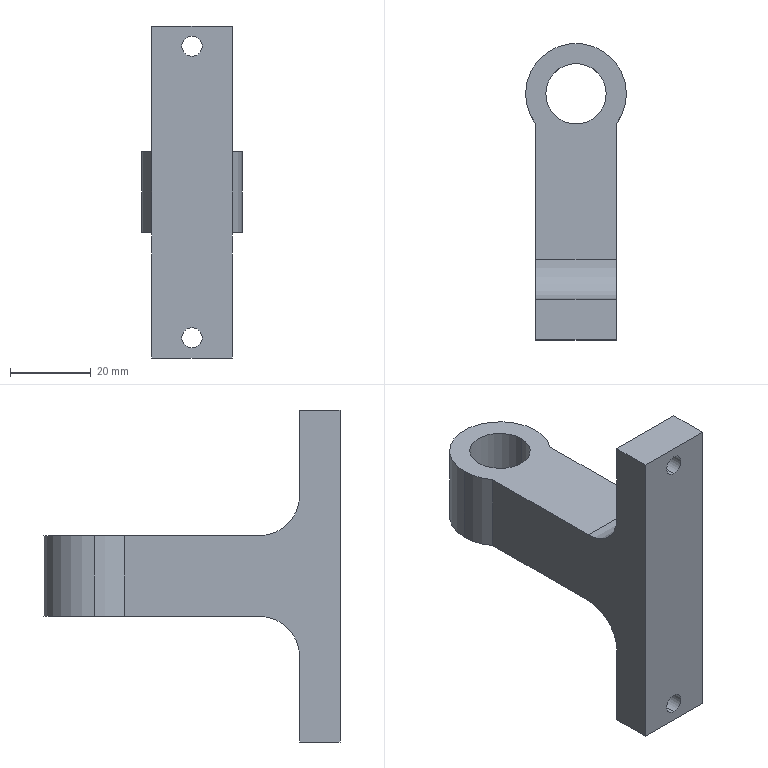Part | SolidWorks | features ICE 2, 3DProfileFeature 1, Extrusion 1, HoleWzd 1, MirrorPattern 1 | 1 solid | 20 faces | box 25 x 73.5 x 82.337 mm | volume 39218 mm3 | cylinder 11 | plane 9 | commonest cylinder face diameters 5 x4 25 x3 15 x2 20 x2
STEP:
#1=CARTESIAN_POINT('',(0.,-61.,-38.668));
#2=VERTEX_POINT('',#1);
#3=CARTESIAN_POINT('',(0.,-61.,-33.668));
#4=VERTEX_POINT('',#3);
#5=CARTESIAN_POINT('',(0.,-61.,-36.168));
#6=DIRECTION('',(0.,1.,0.));
#7=DIRECTION('',(0.,0.,1.));
#8=AXIS2_PLACEMENT_3D('',#5,#6,#7);
#9=CIRCLE('',#8,2.5);
#10=EDGE_CURVE('',#2,#4,#9,.T.);
#11=ORIENTED_EDGE('',*,*,#10,.F.);
#12=CARTESIAN_POINT('',(0.,-51.,-38.668));
#13=VERTEX_POINT('',#12);
#14=CARTESIAN_POINT('',(0.,-51.,-38.668));
#15=DIRECTION('',(0.,1.,0.));
#16=VECTOR('',#15,1000.);
#17=LINE('',#14,#16);
#18=EDGE_CURVE('',#2,#13,#17,.T.);
#19=ORIENTED_EDGE('',*,*,#18,.T.);
#20=CARTESIAN_POINT('',(0.,-51.,-33.668));
#21=VERTEX_POINT('',#20);
#22=CARTESIAN_POINT('',(0.,-51.,-36.168));
#23=DIRECTION('',(0.,1.,0.));
#24=DIRECTION('',(0.,0.,1.));
#25=AXIS2_PLACEMENT_3D('',#22,#23,#24);
#26=CIRCLE('',#25,2.5);
#27=EDGE_CURVE('',#13,#21,#26,.T.);
#28=ORIENTED_EDGE('',*,*,#27,.T.);
#29=CARTESIAN_POINT('',(0.,-51.,-33.668));
#30=DIRECTION('',(0.,1.,0.));
#31=VECTOR('',#30,1000.);
#32=LINE('',#29,#31);
#33=EDGE_CURVE('',#4,#21,#32,.T.);
#34=ORIENTED_EDGE('',*,*,#33,.F.);
#35=EDGE_LOOP('',(#11,#19,#28,#34));
#36=FACE_OUTER_BOUND('',#35,.T.);
#37=CARTESIAN_POINT('',(0.,-51.,-36.168));
#38=DIRECTION('',(0.,1.,0.));
#39=DIRECTION('',(0.,0.,1.));
#40=AXIS2_PLACEMENT_3D('',#37,#38,#39);
#41=CYLINDRICAL_SURFACE('',#40,2.5);
#42=ADVANCED_FACE('',(#36),#41,.F.);
#43=CARTESIAN_POINT('',(0.,-61.,33.668));
#44=VERTEX_POINT('',#43);
#45=CARTESIAN_POINT('',(0.,-61.,38.668));
#46=VERTEX_POINT('',#45);
#47=CARTESIAN_POINT('',(0.,-61.,36.168));
#48=DIRECTION('',(0.,1.,0.));
#49=DIRECTION('',(0.,0.,1.));
#50=AXIS2_PLACEMENT_3D('',#47,#48,#49);
#51=CIRCLE('',#50,2.5);
#52=EDGE_CURVE('',#44,#46,#51,.T.);
#53=ORIENTED_EDGE('',*,*,#52,.F.);
#54=CARTESIAN_POINT('',(0.,-51.,33.668));
#55=VERTEX_POINT('',#54);
#56=CARTESIAN_POINT('',(0.,-51.,33.668));
#57=DIRECTION('',(0.,1.,0.));
#58=VECTOR('',#57,1000.);
#59=LINE('',#56,#58);
#60=EDGE_CURVE('',#44,#55,#59,.T.);
#61=ORIENTED_EDGE('',*,*,#60,.T.);
#62=CARTESIAN_POINT('',(0.,-51.,38.668));
#63=VERTEX_POINT('',#62);
#64=CARTESIAN_POINT('',(0.,-51.,36.168));
#65=DIRECTION('',(0.,1.,0.));
#66=DIRECTION('',(0.,0.,1.));
#67=AXIS2_PLACEMENT_3D('',#64,#65,#66);
#68=CIRCLE('',#67,2.5);
#69=EDGE_CURVE('',#55,#63,#68,.T.);
#70=ORIENTED_EDGE('',*,*,#69,.T.);
#71=CARTESIAN_POINT('',(0.,-51.,38.668));
#72=DIRECTION('',(0.,1.,0.));
#73=VECTOR('',#72,1000.);
#74=LINE('',#71,#73);
#75=EDGE_CURVE('',#46,#63,#74,.T.);
#76=ORIENTED_EDGE('',*,*,#75,.F.);
#77=EDGE_LOOP('',(#53,#61,#70,#76));
#78=FACE_OUTER_BOUND('',#77,.T.);
#79=CARTESIAN_POINT('',(0.,-51.,36.168));
#80=DIRECTION('',(0.,1.,0.));
#81=DIRECTION('',(0.,0.,1.));
#82=AXIS2_PLACEMENT_3D('',#79,#80,#81);
#83=CYLINDRICAL_SURFACE('',#82,2.5);
#84=ADVANCED_FACE('',(#78),#83,.F.);
#85=CARTESIAN_POINT('',(-7.5,0.,10.));
#86=VERTEX_POINT('',#85);
#87=CARTESIAN_POINT('',(7.5,0.,10.));
#88=VERTEX_POINT('',#87);
#89=CARTESIAN_POINT('',(0.,0.,10.));
#90=DIRECTION('',(0.,0.,1.));
#91=DIRECTION('',(1.,0.,0.));
#92=AXIS2_PLACEMENT_3D('',#89,#90,#91);
#93=CIRCLE('',#92,7.5);
#94=EDGE_CURVE('',#86,#88,#93,.T.);
#95=ORIENTED_EDGE('',*,*,#94,.T.);
#96=CARTESIAN_POINT('',(7.5,0.,-10.));
#97=VERTEX_POINT('',#96);
#98=CARTESIAN_POINT('',(7.5,0.,10.));
#99=DIRECTION('',(0.,0.,-1.));
#100=VECTOR('',#99,1000.);
#101=LINE('',#98,#100);
#102=EDGE_CURVE('',#88,#97,#101,.T.);
#103=ORIENTED_EDGE('',*,*,#102,.T.);
#104=CARTESIAN_POINT('',(-7.5,0.,-10.));
#105=VERTEX_POINT('',#104);
#106=CARTESIAN_POINT('',(0.,0.,-10.));
#107=DIRECTION('',(0.,0.,1.));
#108=DIRECTION('',(1.,0.,0.));
#109=AXIS2_PLACEMENT_3D('',#106,#107,#108);
#110=CIRCLE('',#109,7.5);
#111=EDGE_CURVE('',#105,#97,#110,.T.);
#112=ORIENTED_EDGE('',*,*,#111,.F.);
#113=CARTESIAN_POINT('',(-7.5,0.,10.));
#114=DIRECTION('',(0.,0.,-1.));
#115=VECTOR('',#114,1000.);
#116=LINE('',#113,#115);
#117=EDGE_CURVE('',#86,#105,#116,.T.);
#118=ORIENTED_EDGE('',*,*,#117,.F.);
#119=EDGE_LOOP('',(#95,#103,#112,#118));
#120=FACE_OUTER_BOUND('',#119,.T.);
#121=CARTESIAN_POINT('',(0.,0.,10.));
#122=DIRECTION('',(0.,0.,-1.));
#123=DIRECTION('',(-1.,0.,0.));
#124=AXIS2_PLACEMENT_3D('',#121,#122,#123);
#125=CYLINDRICAL_SURFACE('',#124,7.5);
#126=ADVANCED_FACE('',(#120),#125,.F.);
#127=CARTESIAN_POINT('',(12.5,0.,10.));
#128=VERTEX_POINT('',#127);
#129=CARTESIAN_POINT('',(-12.5,0.,10.));
#130=VERTEX_POINT('',#129);
#131=CARTESIAN_POINT('',(0.,0.,10.));
#132=DIRECTION('',(0.,0.,1.));
#133=DIRECTION('',(1.,0.,0.));
#134=AXIS2_PLACEMENT_3D('',#131,#132,#133);
#135=CIRCLE('',#134,12.5);
#136=EDGE_CURVE('',#128,#130,#135,.T.);
#137=ORIENTED_EDGE('',*,*,#136,.F.);
#138=CARTESIAN_POINT('',(12.5,0.,-10.));
#139=VERTEX_POINT('',#138);
#140=CARTESIAN_POINT('',(12.5,0.,10.));
#141=DIRECTION('',(0.,0.,-1.));
#142=VECTOR('',#141,1000.);
#143=LINE('',#140,#142);
#144=EDGE_CURVE('',#128,#139,#143,.T.);
#145=ORIENTED_EDGE('',*,*,#144,.T.);
#146=CARTESIAN_POINT('',(-12.5,0.,-10.));
#147=VERTEX_POINT('',#146);
#148=CARTESIAN_POINT('',(0.,0.,-10.));
#149=DIRECTION('',(0.,0.,1.));
#150=DIRECTION('',(1.,0.,0.));
#151=AXIS2_PLACEMENT_3D('',#148,#149,#150);
#152=CIRCLE('',#151,12.5);
#153=EDGE_CURVE('',#139,#147,#152,.T.);
#154=ORIENTED_EDGE('',*,*,#153,.T.);
#155=CARTESIAN_POINT('',(-12.5,0.,10.));
#156=DIRECTION('',(0.,0.,-1.));
#157=VECTOR('',#156,1000.);
#158=LINE('',#155,#157);
#159=EDGE_CURVE('',#130,#147,#158,.T.);
#160=ORIENTED_EDGE('',*,*,#159,.F.);
#161=EDGE_LOOP('',(#137,#145,#154,#160));
#162=FACE_OUTER_BOUND('',#161,.T.);
#163=CARTESIAN_POINT('',(0.,0.,10.));
#164=DIRECTION('',(0.,0.,-1.));
#165=DIRECTION('',(-1.,0.,0.));
#166=AXIS2_PLACEMENT_3D('',#163,#164,#165);
#167=CYLINDRICAL_SURFACE('',#166,12.5);
#168=ADVANCED_FACE('',(#162),#167,.T.);
#169=CARTESIAN_POINT('',(-10.,-7.5,10.));
#170=VERTEX_POINT('',#169);
#171=CARTESIAN_POINT('',(0.,0.,10.));
#172=DIRECTION('',(0.,0.,1.));
#173=DIRECTION('',(1.,0.,0.));
#174=AXIS2_PLACEMENT_3D('',#171,#172,#173);
#175=CIRCLE('',#174,12.5);
#176=EDGE_CURVE('',#130,#170,#175,.T.);
#177=ORIENTED_EDGE('',*,*,#176,.F.);
#178=ORIENTED_EDGE('',*,*,#159,.T.);
#179=CARTESIAN_POINT('',(-10.,-7.5,-10.));
#180=VERTEX_POINT('',#179);
#181=CARTESIAN_POINT('',(0.,0.,-10.));
#182=DIRECTION('',(0.,0.,1.));
#183=DIRECTION('',(1.,0.,0.));
#184=AXIS2_PLACEMENT_3D('',#181,#182,#183);
#185=CIRCLE('',#184,12.5);
#186=EDGE_CURVE('',#147,#180,#185,.T.);
#187=ORIENTED_EDGE('',*,*,#186,.T.);
#188=CARTESIAN_POINT('',(-10.,-7.5,10.));
#189=DIRECTION('',(0.,0.,1.));
#190=VECTOR('',#189,1000.);
#191=LINE('',#188,#190);
#192=EDGE_CURVE('',#180,#170,#191,.T.);
#193=ORIENTED_EDGE('',*,*,#192,.T.);
#194=EDGE_LOOP('',(#177,#178,#187,#193));
#195=FACE_OUTER_BOUND('',#194,.T.);
#196=CARTESIAN_POINT('',(0.,0.,10.));
#197=DIRECTION('',(0.,0.,-1.));
#198=DIRECTION('',(-1.,0.,0.));
#199=AXIS2_PLACEMENT_3D('',#196,#197,#198);
#200=CYLINDRICAL_SURFACE('',#199,12.5);
#201=ADVANCED_FACE('',(#195),#200,.T.);
#202=CARTESIAN_POINT('',(-10.,-51.,-41.168));
#203=VERTEX_POINT('',#202);
#204=CARTESIAN_POINT('',(-10.,-51.,-20.));
#205=VERTEX_POINT('',#204);
#206=CARTESIAN_POINT('',(-10.,-51.,-20.));
#207=DIRECTION('',(0.,0.,1.));
#208=VECTOR('',#207,1000.);
#209=LINE('',#206,#208);
#210=EDGE_CURVE('',#203,#205,#209,.T.);
#211=ORIENTED_EDGE('',*,*,#210,.T.);
#212=CARTESIAN_POINT('',(10.,-51.,-20.));
#213=VERTEX_POINT('',#212);
#214=CARTESIAN_POINT('',(10.,-51.,-20.));
#215=DIRECTION('',(-1.,0.,0.));
#216=VECTOR('',#215,1000.);
#217=LINE('',#214,#216);
#218=EDGE_CURVE('',#213,#205,#217,.T.);
#219=ORIENTED_EDGE('',*,*,#218,.F.);
#220=CARTESIAN_POINT('',(10.,-51.,-41.168));
#221=VERTEX_POINT('',#220);
#222=CARTESIAN_POINT('',(10.,-51.,-21.658));
#223=DIRECTION('',(0.,0.,1.));
#224=VECTOR('',#223,1000.);
#225=LINE('',#222,#224);
#226=EDGE_CURVE('',#221,#213,#225,.T.);
#227=ORIENTED_EDGE('',*,*,#226,.F.);
#228=CARTESIAN_POINT('',(10.,-51.,-41.168));
#229=DIRECTION('',(-1.,0.,0.));
#230=VECTOR('',#229,1000.);
#231=LINE('',#228,#230);
#232=EDGE_CURVE('',#221,#203,#231,.T.);
#233=ORIENTED_EDGE('',*,*,#232,.T.);
#234=EDGE_LOOP('',(#211,#219,#227,#233));
#235=FACE_OUTER_BOUND('',#234,.T.);
#236=CARTESIAN_POINT('',(0.,-51.,-36.168));
#237=DIRECTION('',(0.,1.,0.));
#238=DIRECTION('',(0.,0.,1.));
#239=AXIS2_PLACEMENT_3D('',#236,#237,#238);
#240=CIRCLE('',#239,2.5);
#241=EDGE_CURVE('',#21,#13,#240,.T.);
#242=ORIENTED_EDGE('',*,*,#241,.F.);
#243=ORIENTED_EDGE('',*,*,#27,.F.);
#244=EDGE_LOOP('',(#242,#243));
#245=FACE_BOUND('',#244,.T.);
#246=CARTESIAN_POINT('',(10.,-51.,-20.));
#247=DIRECTION('',(0.,-1.,0.));
#248=DIRECTION('',(0.,0.,-1.));
#249=AXIS2_PLACEMENT_3D('',#246,#247,#248);
#250=PLANE('',#249);
#251=ADVANCED_FACE('',(#235,#245),#250,.F.);
#252=ORIENTED_EDGE('',*,*,#144,.F.);
#253=CARTESIAN_POINT('',(10.,-7.5,10.));
#254=VERTEX_POINT('',#253);
#255=CARTESIAN_POINT('',(0.,0.,10.));
#256=DIRECTION('',(0.,0.,1.));
#257=DIRECTION('',(1.,0.,0.));
#258=AXIS2_PLACEMENT_3D('',#255,#256,#257);
#259=CIRCLE('',#258,12.5);
#260=EDGE_CURVE('',#254,#128,#259,.T.);
#261=ORIENTED_EDGE('',*,*,#260,.F.);
#262=CARTESIAN_POINT('',(10.,-7.5,-10.));
#263=VERTEX_POINT('',#262);
#264=CARTESIAN_POINT('',(10.,-7.5,10.));
#265=DIRECTION('',(0.,0.,-1.));
#266=VECTOR('',#265,1000.);
#267=LINE('',#264,#266);
#268=EDGE_CURVE('',#254,#263,#267,.T.);
#269=ORIENTED_EDGE('',*,*,#268,.T.);
#270=CARTESIAN_POINT('',(0.,0.,-10.));
#271=DIRECTION('',(0.,0.,1.));
#272=DIRECTION('',(1.,0.,0.));
#273=AXIS2_PLACEMENT_3D('',#270,#271,#272);
#274=CIRCLE('',#273,12.5);
#275=EDGE_CURVE('',#263,#139,#274,.T.);
#276=ORIENTED_EDGE('',*,*,#275,.T.);
#277=EDGE_LOOP('',(#252,#261,#269,#276));
#278=FACE_OUTER_BOUND('',#277,.T.);
#279=CARTESIAN_POINT('',(0.,0.,10.));
#280=DIRECTION('',(0.,0.,-1.));
#281=DIRECTION('',(-1.,0.,0.));
#282=AXIS2_PLACEMENT_3D('',#279,#280,#281);
#283=CYLINDRICAL_SURFACE('',#282,12.5);
#284=ADVANCED_FACE('',(#278),#283,.T.);
#285=CARTESIAN_POINT('',(10.,-41.,10.));
#286=VERTEX_POINT('',#285);
#287=CARTESIAN_POINT('',(10.,-12.5,10.));
#288=DIRECTION('',(0.,-1.,0.));
#289=VECTOR('',#288,1000.);
#290=LINE('',#287,#289);
#291=EDGE_CURVE('',#254,#286,#290,.T.);
#292=ORIENTED_EDGE('',*,*,#291,.F.);
#293=ORIENTED_EDGE('',*,*,#260,.T.);
#294=ORIENTED_EDGE('',*,*,#136,.T.);
#295=ORIENTED_EDGE('',*,*,#176,.T.);
#296=CARTESIAN_POINT('',(-10.,-41.,10.));
#297=VERTEX_POINT('',#296);
#298=CARTESIAN_POINT('',(-10.,12.501,10.));
#299=DIRECTION('',(0.,-1.,0.));
#300=VECTOR('',#299,1000.);
#301=LINE('',#298,#300);
#302=EDGE_CURVE('',#170,#297,#301,.T.);
#303=ORIENTED_EDGE('',*,*,#302,.T.);
#304=CARTESIAN_POINT('',(10.,-41.,10.));
#305=DIRECTION('',(-1.,0.,0.));
#306=VECTOR('',#305,1000.);
#307=LINE('',#304,#306);
#308=EDGE_CURVE('',#286,#297,#307,.T.);
#309=ORIENTED_EDGE('',*,*,#308,.F.);
#310=EDGE_LOOP('',(#292,#293,#294,#295,#303,#309));
#311=FACE_OUTER_BOUND('',#310,.T.);
#312=ORIENTED_EDGE('',*,*,#94,.F.);
#313=CARTESIAN_POINT('',(0.,0.,10.));
#314=DIRECTION('',(0.,0.,1.));
#315=DIRECTION('',(1.,0.,0.));
#316=AXIS2_PLACEMENT_3D('',#313,#314,#315);
#317=CIRCLE('',#316,7.5);
#318=EDGE_CURVE('',#88,#86,#317,.T.);
#319=ORIENTED_EDGE('',*,*,#318,.F.);
#320=EDGE_LOOP('',(#312,#319));
#321=FACE_BOUND('',#320,.T.);
#322=CARTESIAN_POINT('',(0.,0.,10.));
#323=DIRECTION('',(0.,0.,1.));
#324=DIRECTION('',(1.,0.,0.));
#325=AXIS2_PLACEMENT_3D('',#322,#323,#324);
#326=PLANE('',#325);
#327=ADVANCED_FACE('',(#311,#321),#326,.T.);
#328=ORIENTED_EDGE('',*,*,#275,.F.);
#329=CARTESIAN_POINT('',(10.,-41.,-10.));
#330=VERTEX_POINT('',#329);
#331=CARTESIAN_POINT('',(10.,-12.5,-10.));
#332=DIRECTION('',(0.,1.,0.));
#333=VECTOR('',#332,1000.);
#334=LINE('',#331,#333);
#335=EDGE_CURVE('',#330,#263,#334,.T.);
#336=ORIENTED_EDGE('',*,*,#335,.F.);
#337=CARTESIAN_POINT('',(-10.,-41.,-10.));
#338=VERTEX_POINT('',#337);
#339=CARTESIAN_POINT('',(10.,-41.,-10.));
#340=DIRECTION('',(-1.,0.,0.));
#341=VECTOR('',#340,1000.);
#342=LINE('',#339,#341);
#343=EDGE_CURVE('',#330,#338,#342,.T.);
#344=ORIENTED_EDGE('',*,*,#343,.T.);
#345=CARTESIAN_POINT('',(-10.,12.501,-10.));
#346=DIRECTION('',(0.,-1.,0.));
#347=VECTOR('',#346,1000.);
#348=LINE('',#345,#347);
#349=EDGE_CURVE('',#180,#338,#348,.T.);
#350=ORIENTED_EDGE('',*,*,#349,.F.);
#351=ORIENTED_EDGE('',*,*,#186,.F.);
#352=ORIENTED_EDGE('',*,*,#153,.F.);
#353=EDGE_LOOP('',(#328,#336,#344,#350,#351,#352));
#354=FACE_OUTER_BOUND('',#353,.T.);
#355=ORIENTED_EDGE('',*,*,#111,.T.);
#356=CARTESIAN_POINT('',(0.,0.,-10.));
#357=DIRECTION('',(0.,0.,1.));
#358=DIRECTION('',(1.,0.,0.));
#359=AXIS2_PLACEMENT_3D('',#356,#357,#358);
#360=CIRCLE('',#359,7.5);
#361=EDGE_CURVE('',#97,#105,#360,.T.);
#362=ORIENTED_EDGE('',*,*,#361,.T.);
#363=EDGE_LOOP('',(#355,#362));
#364=FACE_BOUND('',#363,.T.);
#365=CARTESIAN_POINT('',(0.,0.,-10.));
#366=DIRECTION('',(0.,0.,1.));
#367=DIRECTION('',(1.,0.,0.));
#368=AXIS2_PLACEMENT_3D('',#365,#366,#367);
#369=PLANE('',#368);
#370=ADVANCED_FACE('',(#354,#364),#369,.F.);
#371=ORIENTED_EDGE('',*,*,#102,.F.);
#372=ORIENTED_EDGE('',*,*,#318,.T.);
#373=ORIENTED_EDGE('',*,*,#117,.T.);
#374=ORIENTED_EDGE('',*,*,#361,.F.);
#375=EDGE_LOOP('',(#371,#372,#373,#374));
#376=FACE_OUTER_BOUND('',#375,.T.);
#377=CARTESIAN_POINT('',(0.,0.,10.));
#378=DIRECTION('',(0.,0.,-1.));
#379=DIRECTION('',(-1.,0.,0.));
#380=AXIS2_PLACEMENT_3D('',#377,#378,#379);
#381=CYLINDRICAL_SURFACE('',#380,7.5);
#382=ADVANCED_FACE('',(#376),#381,.F.);
#383=ORIENTED_EDGE('',*,*,#192,.F.);
#384=ORIENTED_EDGE('',*,*,#349,.T.);
#385=CARTESIAN_POINT('',(-10.,-41.,-20.));
#386=DIRECTION('',(-1.,0.,0.));
#387=DIRECTION('',(0.,0.,1.));
#388=AXIS2_PLACEMENT_3D('',#385,#386,#387);
#389=CIRCLE('',#388,10.);
#390=EDGE_CURVE('',#205,#338,#389,.T.);
#391=ORIENTED_EDGE('',*,*,#390,.F.);
#392=ORIENTED_EDGE('',*,*,#210,.F.);
#393=CARTESIAN_POINT('',(-10.,-61.,-41.168));
#394=VERTEX_POINT('',#393);
#395=CARTESIAN_POINT('',(-10.,-51.,-41.168));
#396=DIRECTION('',(0.,1.,0.));
#397=VECTOR('',#396,1000.);
#398=LINE('',#395,#397);
#399=EDGE_CURVE('',#394,#203,#398,.T.);
#400=ORIENTED_EDGE('',*,*,#399,.F.);
#401=CARTESIAN_POINT('',(-10.,-61.,41.168));
#402=VERTEX_POINT('',#401);
#403=CARTESIAN_POINT('',(-10.,-61.,-41.168));
#404=DIRECTION('',(0.,0.,-1.));
#405=VECTOR('',#404,1000.);
#406=LINE('',#403,#405);
#407=EDGE_CURVE('',#402,#394,#406,.T.);
#408=ORIENTED_EDGE('',*,*,#407,.F.);
#409=CARTESIAN_POINT('',(-10.,-51.,41.168));
#410=VERTEX_POINT('',#409);
#411=CARTESIAN_POINT('',(-10.,-51.,41.168));
#412=DIRECTION('',(0.,-1.,0.));
#413=VECTOR('',#412,1000.);
#414=LINE('',#411,#413);
#415=EDGE_CURVE('',#410,#402,#414,.T.);
#416=ORIENTED_EDGE('',*,*,#415,.F.);
#417=CARTESIAN_POINT('',(-10.,-51.,20.));
#418=VERTEX_POINT('',#417);
#419=CARTESIAN_POINT('',(-10.,-51.,21.658));
#420=DIRECTION('',(0.,0.,1.));
#421=VECTOR('',#420,1000.);
#422=LINE('',#419,#421);
#423=EDGE_CURVE('',#418,#410,#422,.T.);
#424=ORIENTED_EDGE('',*,*,#423,.F.);
#425=CARTESIAN_POINT('',(-10.,-41.,20.));
#426=DIRECTION('',(-1.,0.,0.));
#427=DIRECTION('',(0.,0.,-1.));
#428=AXIS2_PLACEMENT_3D('',#425,#426,#427);
#429=CIRCLE('',#428,10.);
#430=EDGE_CURVE('',#297,#418,#429,.T.);
#431=ORIENTED_EDGE('',*,*,#430,.F.);
#432=ORIENTED_EDGE('',*,*,#302,.F.);
#433=EDGE_LOOP('',(#383,#384,#391,#392,#400,#408,#416,#424,#431,#432));
#434=FACE_OUTER_BOUND('',#433,.T.);
#435=CARTESIAN_POINT('',(-10.,12.501,-10.));
#436=DIRECTION('',(1.,0.,0.));
#437=DIRECTION('',(0.,0.,-1.));
#438=AXIS2_PLACEMENT_3D('',#435,#436,#437);
#439=PLANE('',#438);
#440=ADVANCED_FACE('',(#434),#439,.F.);
#441=ORIENTED_EDGE('',*,*,#430,.T.);
#442=CARTESIAN_POINT('',(10.,-51.,20.));
#443=VERTEX_POINT('',#442);
#444=CARTESIAN_POINT('',(10.,-51.,20.));
#445=DIRECTION('',(-1.,0.,0.));
#446=VECTOR('',#445,1000.);
#447=LINE('',#444,#446);
#448=EDGE_CURVE('',#443,#418,#447,.T.);
#449=ORIENTED_EDGE('',*,*,#448,.F.);
#450=CARTESIAN_POINT('',(10.,-41.,20.));
#451=DIRECTION('',(-1.,0.,0.));
#452=DIRECTION('',(0.,0.,-1.));
#453=AXIS2_PLACEMENT_3D('',#450,#451,#452);
#454=CIRCLE('',#453,10.);
#455=EDGE_CURVE('',#286,#443,#454,.T.);
#456=ORIENTED_EDGE('',*,*,#455,.F.);
#457=ORIENTED_EDGE('',*,*,#308,.T.);
#458=EDGE_LOOP('',(#441,#449,#456,#457));
#459=FACE_OUTER_BOUND('',#458,.T.);
#460=CARTESIAN_POINT('',(10.,-41.,20.));
#461=DIRECTION('',(-1.,0.,0.));
#462=DIRECTION('',(0.,0.,1.));
#463=AXIS2_PLACEMENT_3D('',#460,#461,#462);
#464=CYLINDRICAL_SURFACE('',#463,10.);
#465=ADVANCED_FACE('',(#459),#464,.F.);
#466=CARTESIAN_POINT('',(0.,-51.,36.168));
#467=DIRECTION('',(0.,1.,0.));
#468=DIRECTION('',(0.,0.,1.));
#469=AXIS2_PLACEMENT_3D('',#466,#467,#468);
#470=CIRCLE('',#469,2.5);
#471=EDGE_CURVE('',#63,#55,#470,.T.);
#472=ORIENTED_EDGE('',*,*,#471,.F.);
#473=ORIENTED_EDGE('',*,*,#69,.F.);
#474=EDGE_LOOP('',(#472,#473));
#475=FACE_BOUND('',#474,.T.);
#476=ORIENTED_EDGE('',*,*,#423,.T.);
#477=CARTESIAN_POINT('',(10.,-51.,41.168));
#478=VERTEX_POINT('',#477);
#479=CARTESIAN_POINT('',(10.,-51.,41.168));
#480=DIRECTION('',(-1.,0.,0.));
#481=VECTOR('',#480,1000.);
#482=LINE('',#479,#481);
#483=EDGE_CURVE('',#478,#410,#482,.T.);
#484=ORIENTED_EDGE('',*,*,#483,.F.);
#485=CARTESIAN_POINT('',(10.,-51.,20.));
#486=DIRECTION('',(0.,0.,1.));
#487=VECTOR('',#486,1000.);
#488=LINE('',#485,#487);
#489=EDGE_CURVE('',#443,#478,#488,.T.);
#490=ORIENTED_EDGE('',*,*,#489,.F.);
#491=ORIENTED_EDGE('',*,*,#448,.T.);
#492=EDGE_LOOP('',(#476,#484,#490,#491));
#493=FACE_OUTER_BOUND('',#492,.T.);
#494=CARTESIAN_POINT('',(10.,-51.,21.658));
#495=DIRECTION('',(0.,-1.,0.));
#496=DIRECTION('',(0.,0.,-1.));
#497=AXIS2_PLACEMENT_3D('',#494,#495,#496);
#498=PLANE('',#497);
#499=ADVANCED_FACE('',(#475,#493),#498,.F.);
#500=ORIENTED_EDGE('',*,*,#415,.T.);
#501=CARTESIAN_POINT('',(10.,-61.,41.168));
#502=VERTEX_POINT('',#501);
#503=CARTESIAN_POINT('',(10.,-61.,41.168));
#504=DIRECTION('',(-1.,0.,0.));
#505=VECTOR('',#504,1000.);
#506=LINE('',#503,#505);
#507=EDGE_CURVE('',#502,#402,#506,.T.);
#508=ORIENTED_EDGE('',*,*,#507,.F.);
#509=CARTESIAN_POINT('',(10.,-51.,41.168));
#510=DIRECTION('',(0.,-1.,0.));
#511=VECTOR('',#510,1000.);
#512=LINE('',#509,#511);
#513=EDGE_CURVE('',#478,#502,#512,.T.);
#514=ORIENTED_EDGE('',*,*,#513,.F.);
#515=ORIENTED_EDGE('',*,*,#483,.T.);
#516=EDGE_LOOP('',(#500,#508,#514,#515));
#517=FACE_OUTER_BOUND('',#516,.T.);
#518=CARTESIAN_POINT('',(10.,-51.,41.168));
#519=DIRECTION('',(0.,0.,-1.));
#520=DIRECTION('',(-1.,0.,0.));
#521=AXIS2_PLACEMENT_3D('',#518,#519,#520);
#522=PLANE('',#521);
#523=ADVANCED_FACE('',(#517),#522,.F.);
#524=CARTESIAN_POINT('',(0.,-61.,-36.168));
#525=DIRECTION('',(0.,1.,0.));
#526=DIRECTION('',(0.,0.,1.));
#527=AXIS2_PLACEMENT_3D('',#524,#525,#526);
#528=CIRCLE('',#527,2.5);
#529=EDGE_CURVE('',#4,#2,#528,.T.);
#530=ORIENTED_EDGE('',*,*,#529,.T.);
#531=ORIENTED_EDGE('',*,*,#10,.T.);
#532=EDGE_LOOP('',(#530,#531));
#533=FACE_BOUND('',#532,.T.);
#534=CARTESIAN_POINT('',(0.,-61.,36.168));
#535=DIRECTION('',(0.,1.,0.));
#536=DIRECTION('',(0.,0.,1.));
#537=AXIS2_PLACEMENT_3D('',#534,#535,#536);
#538=CIRCLE('',#537,2.5);
#539=EDGE_CURVE('',#46,#44,#538,.T.);
#540=ORIENTED_EDGE('',*,*,#539,.T.);
#541=ORIENTED_EDGE('',*,*,#52,.T.);
#542=EDGE_LOOP('',(#540,#541));
#543=FACE_BOUND('',#542,.T.);
#544=ORIENTED_EDGE('',*,*,#407,.T.);
#545=CARTESIAN_POINT('',(10.,-61.,-41.168));
#546=VERTEX_POINT('',#545);
#547=CARTESIAN_POINT('',(10.,-61.,-41.168));
#548=DIRECTION('',(-1.,0.,0.));
#549=VECTOR('',#548,1000.);
#550=LINE('',#547,#549);
#551=EDGE_CURVE('',#546,#394,#550,.T.);
#552=ORIENTED_EDGE('',*,*,#551,.F.);
#553=CARTESIAN_POINT('',(10.,-61.,-41.168));
#554=DIRECTION('',(0.,0.,-1.));
#555=VECTOR('',#554,1000.);
#556=LINE('',#553,#555);
#557=EDGE_CURVE('',#502,#546,#556,.T.);
#558=ORIENTED_EDGE('',*,*,#557,.F.);
#559=ORIENTED_EDGE('',*,*,#507,.T.);
#560=EDGE_LOOP('',(#544,#552,#558,#559));
#561=FACE_OUTER_BOUND('',#560,.T.);
#562=CARTESIAN_POINT('',(10.,-61.,-41.168));
#563=DIRECTION('',(0.,1.,0.));
#564=DIRECTION('',(0.,0.,1.));
#565=AXIS2_PLACEMENT_3D('',#562,#563,#564);
#566=PLANE('',#565);
#567=ADVANCED_FACE('',(#533,#543,#561),#566,.F.);
#568=ORIENTED_EDGE('',*,*,#399,.T.);
#569=ORIENTED_EDGE('',*,*,#232,.F.);
#570=CARTESIAN_POINT('',(10.,-51.,-41.168));
#571=DIRECTION('',(0.,1.,0.));
#572=VECTOR('',#571,1000.);
#573=LINE('',#570,#572);
#574=EDGE_CURVE('',#546,#221,#573,.T.);
#575=ORIENTED_EDGE('',*,*,#574,.F.);
#576=ORIENTED_EDGE('',*,*,#551,.T.);
#577=EDGE_LOOP('',(#568,#569,#575,#576));
#578=FACE_OUTER_BOUND('',#577,.T.);
#579=CARTESIAN_POINT('',(10.,-51.,-41.168));
#580=DIRECTION('',(0.,0.,1.));
#581=DIRECTION('',(1.,0.,0.));
#582=AXIS2_PLACEMENT_3D('',#579,#580,#581);
#583=PLANE('',#582);
#584=ADVANCED_FACE('',(#578),#583,.F.);
#585=ORIENTED_EDGE('',*,*,#390,.T.);
#586=ORIENTED_EDGE('',*,*,#343,.F.);
#587=CARTESIAN_POINT('',(10.,-41.,-20.));
#588=DIRECTION('',(-1.,0.,0.));
#589=DIRECTION('',(0.,0.,1.));
#590=AXIS2_PLACEMENT_3D('',#587,#588,#589);
#591=CIRCLE('',#590,10.);
#592=EDGE_CURVE('',#213,#330,#591,.T.);
#593=ORIENTED_EDGE('',*,*,#592,.F.);
#594=ORIENTED_EDGE('',*,*,#218,.T.);
#595=EDGE_LOOP('',(#585,#586,#593,#594));
#596=FACE_OUTER_BOUND('',#595,.T.);
#597=CARTESIAN_POINT('',(10.,-41.,-20.));
#598=DIRECTION('',(-1.,0.,0.));
#599=DIRECTION('',(0.,0.,1.));
#600=AXIS2_PLACEMENT_3D('',#597,#598,#599);
#601=CYLINDRICAL_SURFACE('',#600,10.);
#602=ADVANCED_FACE('',(#596),#601,.F.);
#603=ORIENTED_EDGE('',*,*,#335,.T.);
#604=ORIENTED_EDGE('',*,*,#268,.F.);
#605=ORIENTED_EDGE('',*,*,#291,.T.);
#606=ORIENTED_EDGE('',*,*,#455,.T.);
#607=ORIENTED_EDGE('',*,*,#489,.T.);
#608=ORIENTED_EDGE('',*,*,#513,.T.);
#609=ORIENTED_EDGE('',*,*,#557,.T.);
#610=ORIENTED_EDGE('',*,*,#574,.T.);
#611=ORIENTED_EDGE('',*,*,#226,.T.);
#612=ORIENTED_EDGE('',*,*,#592,.T.);
#613=EDGE_LOOP('',(#603,#604,#605,#606,#607,#608,#609,#610,#611,#612));
#614=FACE_OUTER_BOUND('',#613,.T.);
#615=CARTESIAN_POINT('',(10.,-41.,-20.));
#616=DIRECTION('',(-1.,0.,0.));
#617=DIRECTION('',(0.,0.,1.));
#618=AXIS2_PLACEMENT_3D('',#615,#616,#617);
#619=PLANE('',#618);
#620=ADVANCED_FACE('',(#614),#619,.F.);
#621=ORIENTED_EDGE('',*,*,#60,.F.);
#622=ORIENTED_EDGE('',*,*,#539,.F.);
#623=ORIENTED_EDGE('',*,*,#75,.T.);
#624=ORIENTED_EDGE('',*,*,#471,.T.);
#625=EDGE_LOOP('',(#621,#622,#623,#624));
#626=FACE_OUTER_BOUND('',#625,.T.);
#627=CARTESIAN_POINT('',(0.,-51.,36.168));
#628=DIRECTION('',(0.,1.,0.));
#629=DIRECTION('',(0.,0.,1.));
#630=AXIS2_PLACEMENT_3D('',#627,#628,#629);
#631=CYLINDRICAL_SURFACE('',#630,2.5);
#632=ADVANCED_FACE('',(#626),#631,.F.);
#633=ORIENTED_EDGE('',*,*,#18,.F.);
#634=ORIENTED_EDGE('',*,*,#529,.F.);
#635=ORIENTED_EDGE('',*,*,#33,.T.);
#636=ORIENTED_EDGE('',*,*,#241,.T.);
#637=EDGE_LOOP('',(#633,#634,#635,#636));
#638=FACE_OUTER_BOUND('',#637,.T.);
#639=CARTESIAN_POINT('',(0.,-51.,-36.168));
#640=DIRECTION('',(0.,1.,0.));
#641=DIRECTION('',(0.,0.,1.));
#642=AXIS2_PLACEMENT_3D('',#639,#640,#641);
#643=CYLINDRICAL_SURFACE('',#642,2.5);
#644=ADVANCED_FACE('',(#638),#643,.F.);
#645=CLOSED_SHELL('',(#42,#84,#126,#168,#201,#251,#284,#327,#370,#382,#440,#465,#499,#523,#567,#584,#602,#620,#632,#644));
#646=MANIFOLD_SOLID_BREP('',#645);
#647=CARTESIAN_POINT('',(0.,0.,0.));
#648=DIRECTION('',(0.,0.,1.));
#649=DIRECTION('',(1.,0.,0.));
#650=AXIS2_PLACEMENT_3D('',#647,#648,#649);
#651=(LENGTH_UNIT()NAMED_UNIT(*)SI_UNIT(.MILLI.,.METRE.));
#652=UNCERTAINTY_MEASURE_WITH_UNIT(LENGTH_MEASURE(0.00001),#651,'','');
#653=(NAMED_UNIT(*)PLANE_ANGLE_UNIT()SI_UNIT($,.RADIAN.));
#654=(NAMED_UNIT(*)SI_UNIT($,.STERADIAN.)SOLID_ANGLE_UNIT());
#655=(GEOMETRIC_REPRESENTATION_CONTEXT(3)GLOBAL_UNCERTAINTY_ASSIGNED_CONTEXT((#652))GLOBAL_UNIT_ASSIGNED_CONTEXT((#651,#653,#654))REPRESENTATION_CONTEXT('',''));
#656=ADVANCED_BREP_SHAPE_REPRESENTATION('',(#646,#650),#655);